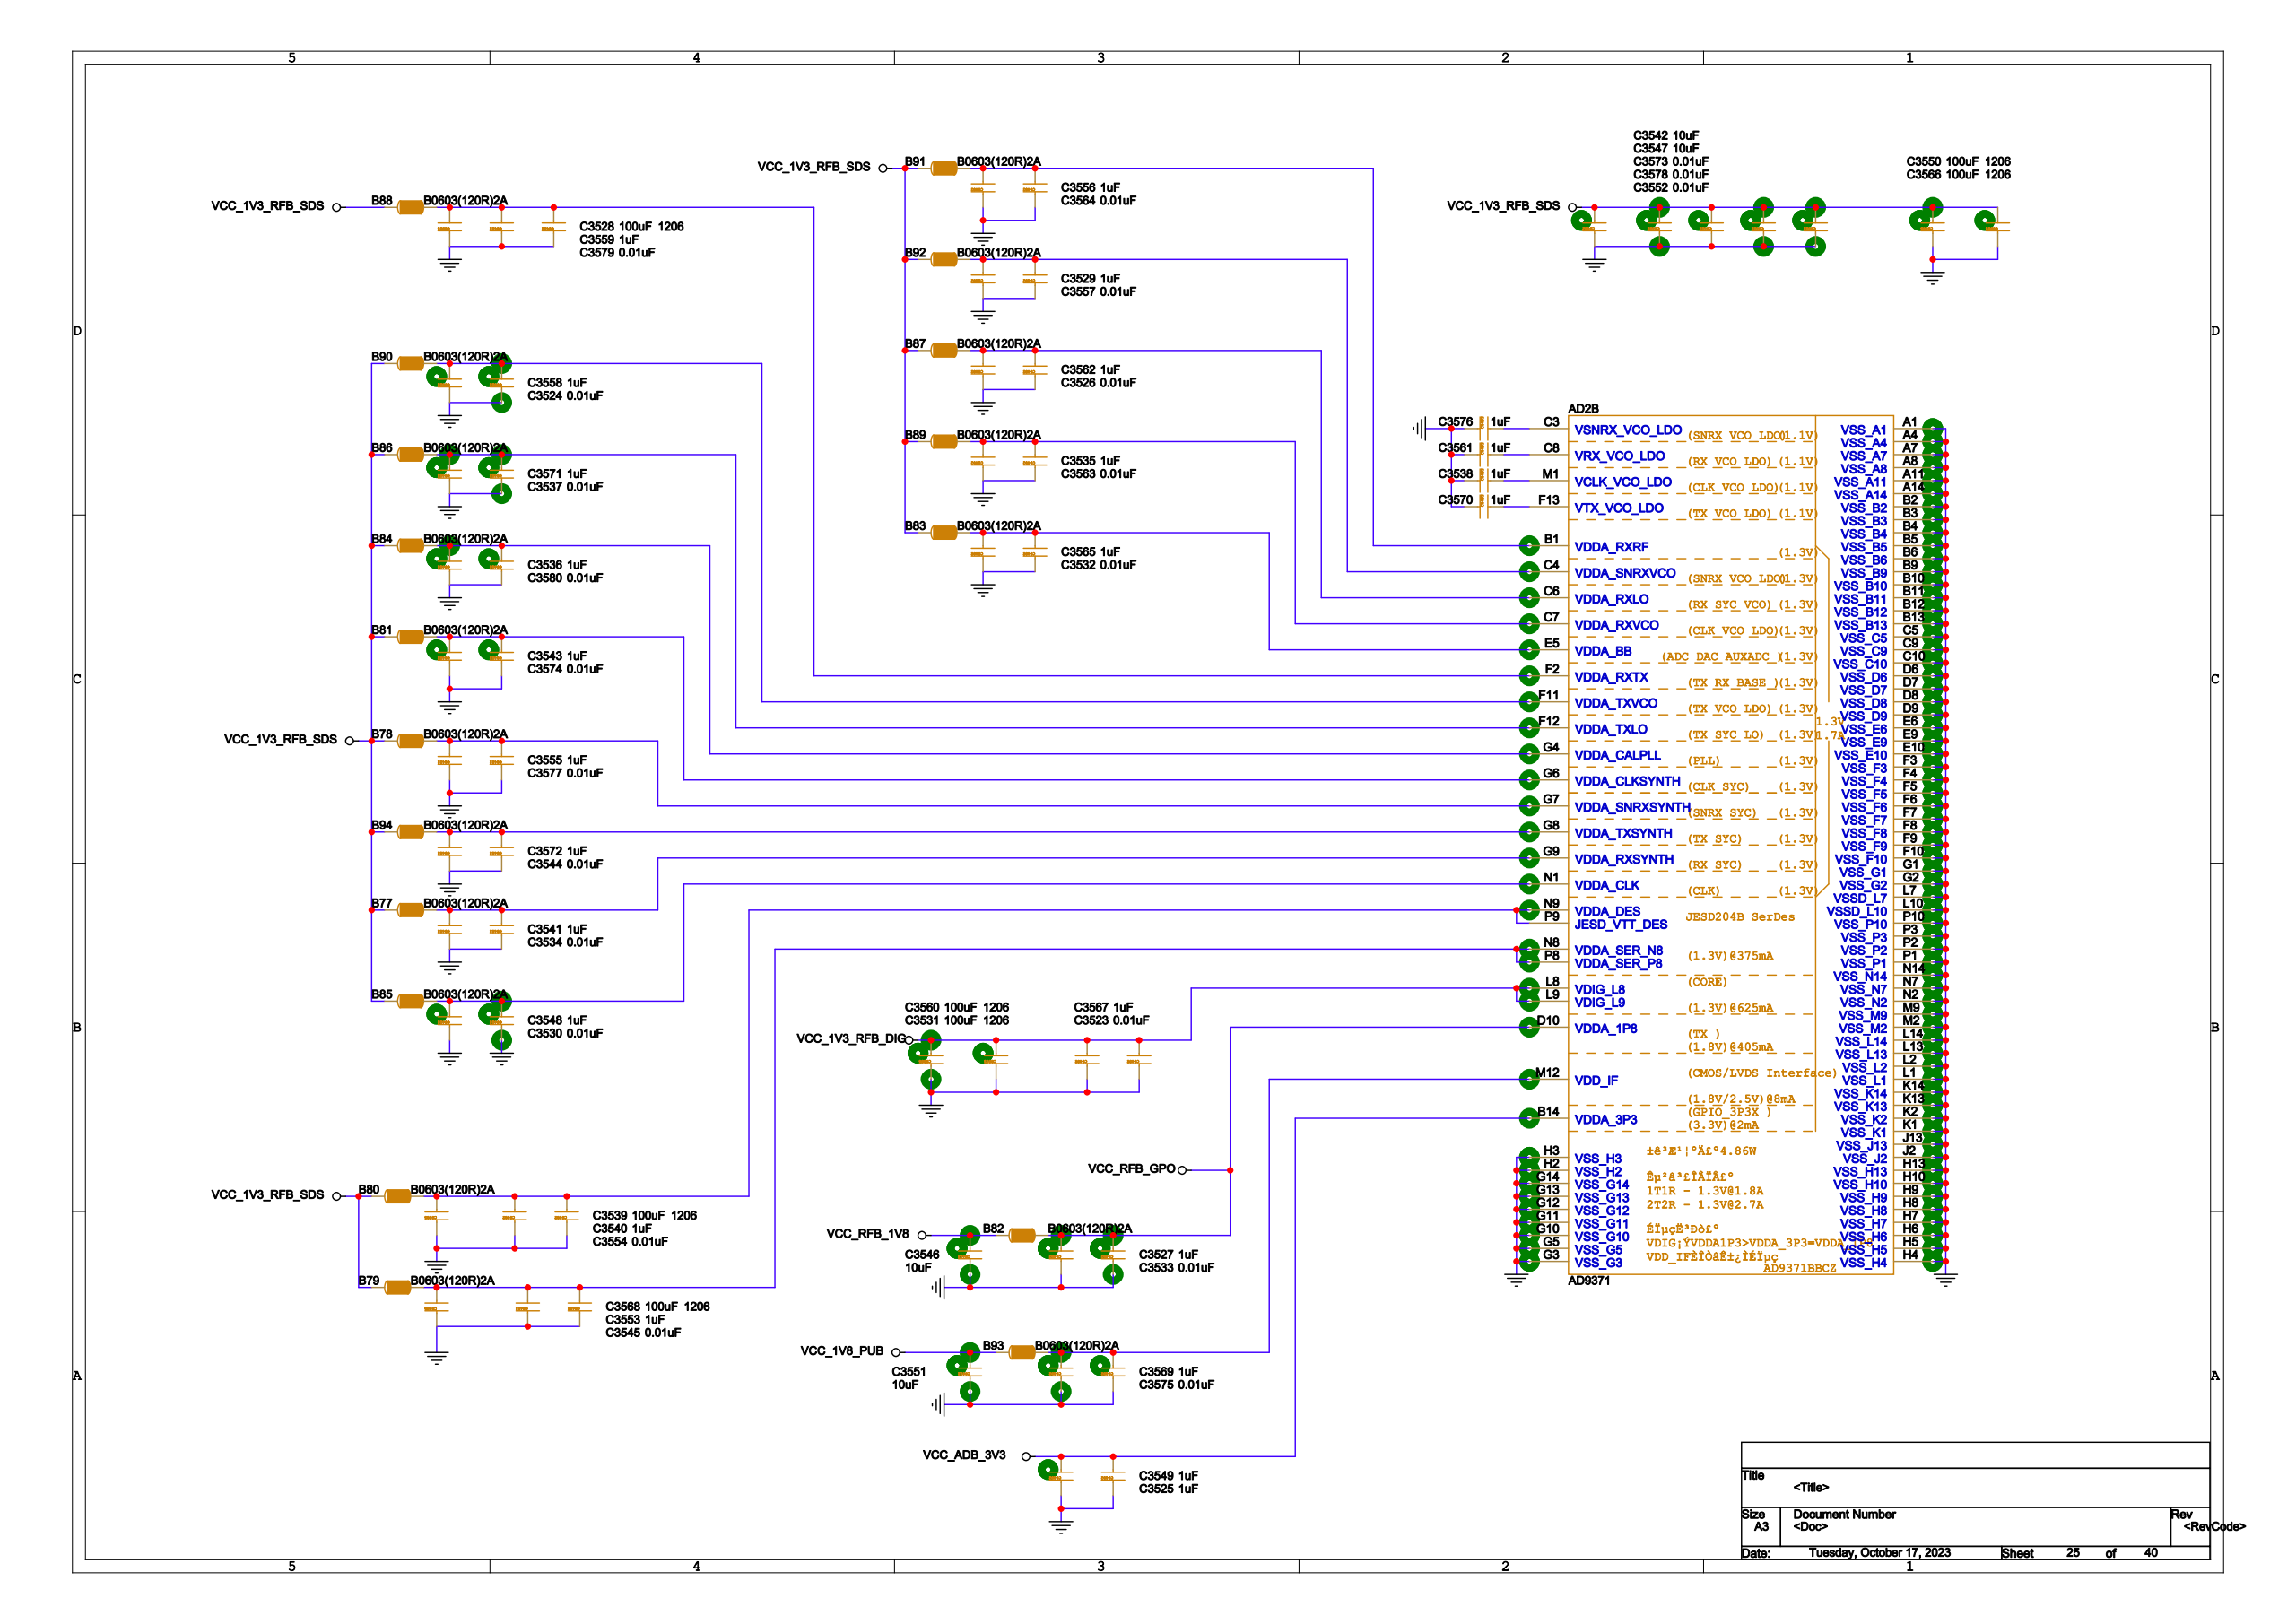Circuit board | Cadence Allegro | 1793 parts | 1223 nets | one sheet of the schematic
Parts on this sheet (reference | value | footprint):
AD2 | AD9371 | BGA196
B77 | B0603(120R)2A | B0603
B78 | B0603(120R)2A | B0603
B79 | B0603(120R)2A | B0603
B80 | B0603(120R)2A | B0603
B81 | B0603(120R)2A | B0603
B82 | B0603(120R)2A | B0603
B83 | B0603(120R)2A | B0603
B84 | B0603(120R)2A | B0603
B85 | B0603(120R)2A | B0603
B86 | B0603(120R)2A | B0603
B87 | B0603(120R)2A | B0603
B88 | B0603(120R)2A | B0603
B89 | B0603(120R)2A | B0603
B90 | B0603(120R)2A | B0603
B91 | B0603(120R)2A | B0603
B92 | B0603(120R)2A | B0603
B93 | B0603(120R)2A | B0603
B94 | B0603(120R)2A | B0603
C3523 | 0.01uF | C0402
C3524 | 0.01uF | C0402
C3525 | 1uF | C0402
C3526 | 0.01uF | C0402
C3527 | 1uF | C0402
C3528 | 100uF | 1206
C3529 | 1uF | C0402
C3530 | 0.01uF | C0402
C3531 | 100uF | 1206
C3532 | 0.01uF | C0402
C3533 | 0.01uF | C0402
C3534 | 0.01uF | C0402
C3535 | 1uF | C0402
C3536 | 1uF | C0402
C3537 | 0.01uF | C0402
C3538 | 1uF | C0402
C3539 | 100uF | 1206
C3540 | 1uF | C0402
C3541 | 1uF | C0402
C3542 | 10uF | C0402
C3543 | 1uF | C0402
C3544 | 0.01uF | C0402
C3545 | 0.01uF | C0402
C3546 | 10uF | C0402
C3547 | 10uF | C0402
C3548 | 1uF | C0402
C3549 | 1uF | C0402
C3550 | 100uF | 1206
C3551 | 10uF | C0402
C3552 | 0.01uF | C0402
C3553 | 1uF | C0402
C3554 | 0.01uF | C0402
C3555 | 1uF | C0402
C3556 | 1uF | C0402
C3557 | 0.01uF | C0402
C3558 | 1uF | C0402
C3559 | 1uF | C0402
C3560 | 100uF | 1206
C3561 | 1uF | C0402
C3562 | 1uF | C0402
C3563 | 0.01uF | C0402
C3564 | 0.01uF | C0402
C3565 | 1uF | C0402
C3566 | 100uF | 1206
C3567 | 1uF | C0402
C3568 | 100uF | 1206
C3569 | 1uF | C0402
C3570 | 1uF | C0402
C3571 | 1uF | C0402
C3572 | 1uF | C0402
C3573 | 0.01uF | C0402
C3574 | 0.01uF | C0402
C3575 | 0.01uF | C0402
C3576 | 1uF | C0402
C3577 | 0.01uF | C0402
C3578 | 0.01uF | C0402
C3579 | 0.01uF | C0402
C3580 | 0.01uF | C0402
Nets of these parts (net: part-pin ...):
GND: C3523-1 C3524-1 C3525-1 C3526-1 C3527-1 C3528-1 C3529-1 C3530-1 C3531-1 C3532-1 C3533-1 C3534-1 C3535-1 C3536-1 C3537-1 C3538-1 C3539-1 C3540-1 C3541-1 C3542-1 C3543-1 C3544-1 C3545-1 C3546-1 C3547-1 C3548-1 C3549-1 C3550-1 C3551-1 C3552-1 C3553-1 C3554-1 C3555-1 C3556-1 C3557-1 C3558-1 C3559-1 C3560-1 C3561-1 C3562-1 C3563-1 C3564-1 C3565-1 C3566-1 C3567-1 C3568-1 C3569-1 C3570-1 C3571-1 C3572-1 C3573-1 C3574-1 C3575-1 C3576-1 C3577-1 C3578-1 C3579-1 C3580-1 AD2-A1 AD2-A4 AD2-A7 AD2-A8 AD2-A11 AD2-A14 AD2-B2 AD2-B3 AD2-B4 AD2-B5 AD2-B6 AD2-B9 AD2-B10 AD2-B11 AD2-B12 AD2-B13 AD2-C5 AD2-C9 AD2-C10 AD2-D6 AD2-D7 AD2-D8 AD2-D9 AD2-E6 AD2-E9 AD2-E10 AD2-F3 AD2-F4 AD2-F5 AD2-F6 AD2-F7 AD2-F8 AD2-F9 AD2-F10 AD2-G1 AD2-G2 AD2-G3 AD2-G5 AD2-G10 AD2-G11 AD2-G12 AD2-G13 AD2-G14 AD2-H2 AD2-H3 AD2-H4 AD2-H5 AD2-H6 AD2-H7 AD2-H8 AD2-H9 AD2-H10 AD2-H13 AD2-J2 AD2-J13 AD2-K1 AD2-K2 AD2-K13 AD2-K14 AD2-L1 AD2-L2 AD2-L7 AD2-L10 AD2-L13 AD2-L14 AD2-M2 AD2-M9 AD2-N2 AD2-N7 AD2-N14 AD2-P1 AD2-P2 AD2-P3 AD2-P10
N17273985: B88-2 C3528-2 C3559-2 C3579-2 AD2-F2
VCC_1V3_RFB_DIG: C3523-2 C3531-2 C3560-2 C3567-2 AD2-L8 AD2-L9
N17273795: B80-2 C3539-2 C3540-2 C3554-2 AD2-N9 AD2-P9
VCC_1V3_RFB_SDS: B77-1 B78-1 B79-1 B80-1 B81-1 B83-1 B84-1 B85-1 B86-1 B87-1 B88-1 B89-1 B90-1 B91-1 B92-1 B94-1 C3542-2 C3547-2 C3550-2 C3552-2 C3566-2 C3573-2 C3578-2
N17273887: B79-2 C3545-2 C3553-2 C3568-2 AD2-N8 AD2-P8
VCC_RFB_1V8: B82-1 C3546-2
VCC_1V8_PUB: B93-1 C3551-2
VCC_ADB_3V3: C3525-2 C3549-2 AD2-B14
N17273857: C3538-2 AD2-M1
VCC_RFB_GPO: B82-2 C3527-2 C3533-2 AD2-D10
N17273973: B83-2 C3532-2 C3565-2 AD2-E5
N17274043: B84-2 C3536-2 C3580-2 AD2-G4
N17274135: B85-2 C3530-2 C3548-2 AD2-N1
N17274057: B81-2 C3543-2 C3574-2 AD2-G6
N17273933: B87-2 C3526-2 C3562-2 AD2-C6
N17273783: B91-2 C3556-2 C3564-2 AD2-B1
N17274107: B77-2 C3534-2 C3541-2 AD2-G9
N17273955: B89-2 C3535-2 C3563-2 AD2-C7
N17274015: B78-2 C3555-2 C3577-2 AD2-G7
N17273879: B92-2 C3529-2 C3557-2 AD2-C4
N17274025: B86-2 C3537-2 C3571-2 AD2-F12
N17274079: B94-2 C3544-2 C3572-2 AD2-G8
N17274005: B90-2 C3524-2 C3558-2 AD2-F11
N17274371: B93-2 C3569-2 C3575-2 AD2-M12
N17273823: C3561-2 AD2-C8
N17273809: C3576-2 AD2-C3
N17273869: C3570-2 AD2-F13